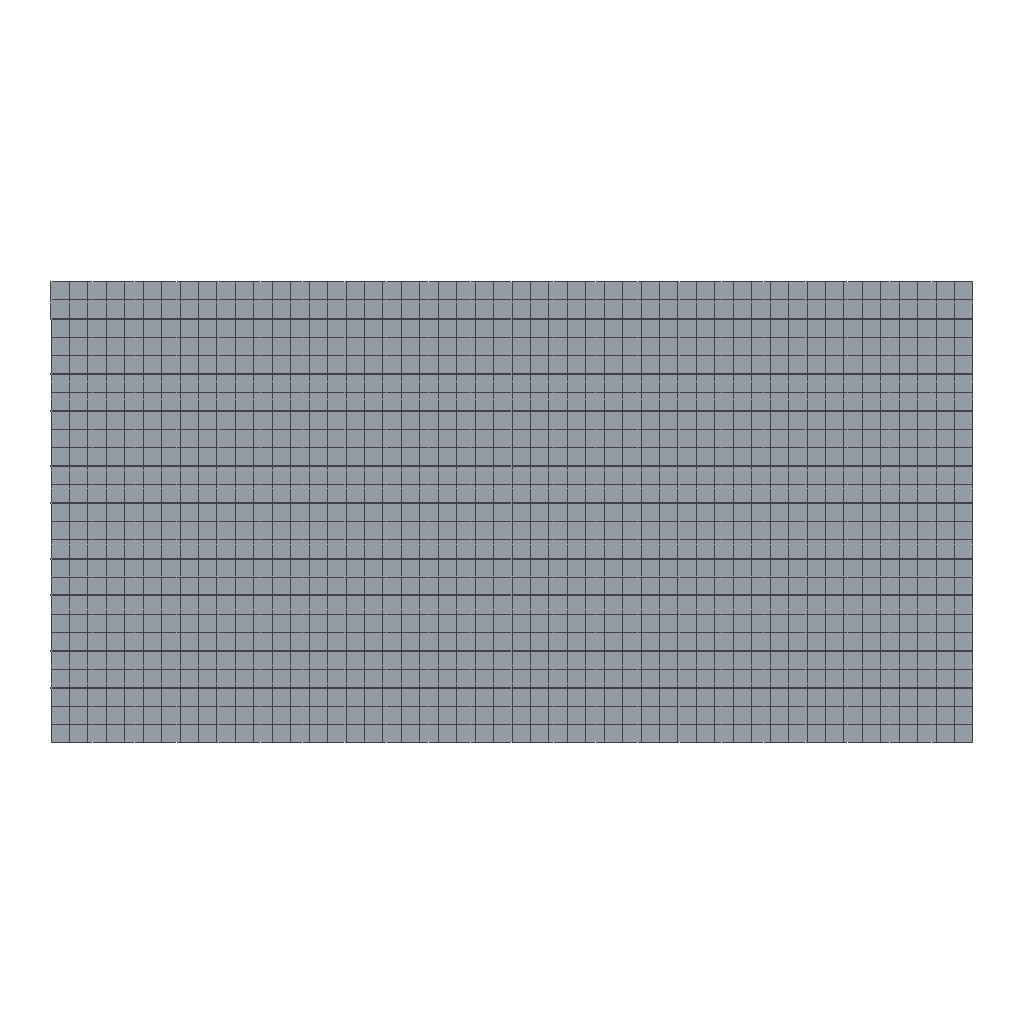Simulation study | abaqus
Set-up summary:
category,name,step,type,value,unit,region
solver,abaqus
solver,version,,,Abaqus/Explicit 2020
units,not stated in the deck,,not stated
analysis,deck,,transient,transient
load_step,Step-1,Step-1,transient
load_step,requested,,,1
mesh,nodes,,,2353
mesh,elements,,,1610
element_type,CPS4R,,plane,1250
element_type,COH2D4,,cohesive,360
load,load commands in deck,,count,1
bc,support commands in deck,,count,4
material,MATERIAL-3,,in results
material,SIC,,in results
material,T300,,in results
check,setup vs results,,match,"per instance, exact: element labels, types and connectivity; labels of the nodes the elements use; coordinates of those nodes at DOUBLE_PRECISION in 1 of 4 instance(s)"
Abaqus input file, long lists of numbers shortened:
*Heading
** Job name: Job-3 Model name: Model-1-Copy
** Generated by: Abaqus/CAE 2020
*Preprint, echo=NO, model=NO, history=NO, contact=NO
**
** PARTS
**
*Part, name=coh
*Node
      1, -0.1, -0.038
      2, -0.1, -0.0382
** (565 more lines like these left out)
*Element, type=COH2D4
 1,   1,  37, 397,  76
 2,  37,   2,  38, 397
** (358 more lines like these left out)
*Nset, nset=Set-1, generate
   1,  567,    1
*Elset, elset=Set-1, generate
   1,  360,    1
** Section: coh
*Cohesive Section, elset=Set-1, controls=EC-1, material=Material-3, response=TRACTION SEPARATION
,
*End Part
**
*Part, name=lay-1
*Node
      1, -0.1, 0.05
      2, -0.1, 0.046
** (151 more lines like these left out)
*Element, type=CPS4R
  1,   1,   2,   5,   4
  2,   2,   3,   6,   5
** (98 more lines like these left out)
*Nset, nset=Set-3, generate
   1,  153,    1
*Elset, elset=Set-3, generate
   1,  100,    1
*Orientation, name=Ori-1
1., 0., 0., 0., 1., 0.
3, 0.
** Section: t300
*Solid Section, elset=Set-3, orientation=Ori-1, material=t300
,
*End Part
**
*Part, name=rigid
*End Part
**
*Part, name=work
*Node
      1,  0.2, -0.0882
      2,           0., -0.0882
** (1630 more lines like these left out)
*Element, type=CPS4R
  1,    1,   37,  947,  138
  2,   37,   38,  948,  947
** (1148 more lines like these left out)
*Nset, nset=Set-2
   29,   30,   31,   32,  743,  744,  745,  746,  747,  748,  749,  750,  751,  752,  753,  754
  755,  756,  757,  758,  759,  760,  761,  762,  763,  764,  765,  766,  767,  768,  769,  770
** (11 more lines like these left out)
*Elset, elset=Set-2, generate
  851,  1000,     1
*Nset, nset=Set-3
   21,   22,   23,   24,  543,  544,  545,  546,  547,  548,  549,  550,  551,  552,  553,  554
  555,  556,  557,  558,  559,  560,  561,  562,  563,  564,  565,  566,  567,  568,  569,  570
** (8 more lines like these left out)
*Elset, elset=Set-3, generate
 651,  750,    1
*Nset, nset=Set-4
   13,   14,   15,   16,  341,  342,  343,  344,  345,  346,  347,  348,  349,  350,  351,  352
  353,  354,  355,  356,  357,  358,  359,  360,  361,  362,  363,  364,  365,  366,  367,  368
** (11 more lines like these left out)
*Elset, elset=Set-4, generate
 401,  550,    1
*Nset, nset=Set-6
    5,    6,    7,    8,  139,  140,  141,  142,  143,  144,  145,  146,  147,  148,  149,  150
  151,  152,  153,  154,  155,  156,  157,  158,  159,  160,  161,  162,  163,  164,  165,  166
** (8 more lines like these left out)
*Elset, elset=Set-6, generate
 151,  250,    1
*Nset, nset=Set-7
    1,    2,    3,    4,    9,   10,   11,   12,   17,   18,   19,   20,   25,   26,   27,   28
   33,   34,   35,   36,   37,   38,   39,   40,   41,   42,   43,   44,   45,   46,   47,   48
** (56 more lines like these left out)
*Elset, elset=Set-7
    1,    2,    3,    4,    5,    6,    7,    8,    9,   10,   11,   12,   13,   14,   15,   16
   17,   18,   19,   20,   21,   22,   23,   24,   25,   26,   27,   28,   29,   30,   31,   32
** (39 more lines like these left out)
*Nset, nset=Set-18
    5,    6,    7,    8,   17,   18,   19,   20,   21,   22,   23,   24,   25,   26,   27,   28
  139,  140,  141,  142,  143,  144,  145,  146,  147,  148,  149,  150,  151,  152,  153,  154
** (37 more lines like these left out)
*Elset, elset=Set-18
 151, 152, 153, 154, 155, 156, 157, 158, 159, 160, 161, 162, 163, 164, 165, 166
 167, 168, 169, 170, 171, 172, 173, 174, 175, 176, 177, 178, 179, 180, 181, 182
** (23 more lines like these left out)
*Nset, nset=Set-19
    1,    2,    3,    4,    9,   10,   11,   12,   13,   14,   15,   16,   29,   30,   31,   32
   33,   34,   35,   36,   37,   38,   39,   40,   41,   42,   43,   44,   45,   46,   47,   48
** (62 more lines like these left out)
*Elset, elset=Set-19
    1,    2,    3,    4,    5,    6,    7,    8,    9,   10,   11,   12,   13,   14,   15,   16
   17,   18,   19,   20,   21,   22,   23,   24,   25,   26,   27,   28,   29,   30,   31,   32
** (45 more lines like these left out)
** Section: sic
*Solid Section, elset=Set-19, material=sic
,
*Orientation, name=Ori-2
1., 0., 0., 0., 1., 0.
3, 0.
** Section: t300
*Solid Section, elset=Set-18, orientation=Ori-2, material=t300
,
*End Part
**
**
** ASSEMBLY
**
*Assembly, name=Assembly
**
*Instance, name=rigid-1, part=rigid
    0.2142,     0.001757,           0.
*Node
      1, 0.005757, -0.01114,           0.
*Nset, nset=rigid-1-RefPt_, internal
1,
*Surface, type=SEGMENTS, name=m_Surf-1
START, 0.01, -0.01
 CIRCL, 0.001515, -0.01, 0.005757, -0.002652
 LINE, -0.04179,        0.015
 LINE, 0.0533,        0.015
 LINE, 0.01, -0.01
*Rigid Body, ref node=rigid-1-RefPt_, analytical surface=m_Surf-1
*End Instance
**
*Instance, name=work-1, part=work
*End Instance
**
*Instance, name=coh-1, part=coh
         0.1,        -0.05,           0.
*End Instance
**
*Instance, name=lay-1-1, part=lay-1
         0.1,        -0.05,           0.
*End Instance
**
*Nset, nset=Set-2, instance=work-1
   3,   4,  88,  89,  90,  91,  92,  93,  94,  95,  96,  97,  98,  99, 100, 101
 102, 103, 104, 105, 106, 107, 108, 109, 110, 111, 112, 113, 114, 115, 116, 117
** (2 more lines like these left out)
*Elset, elset=Set-2, instance=work-1, generate
 101,  150,    1
*Nset, nset=Set-3, instance=work-1
   1,   3,   4,  14,  15,  21,  24,  88,  89,  90,  91,  92,  93,  94,  95,  96
  97,  98,  99, 100, 101, 102, 103, 104, 105, 106, 107, 108, 109, 110, 111, 112
** (2 more lines like these left out)
*Elset, elset=Set-3, instance=work-1
   1,  51, 101, 102, 103, 104, 105, 106, 107, 108, 109, 110, 111, 112, 113, 114
 115, 116, 117, 118, 119, 120, 121, 122, 123, 124, 125, 126, 127, 128, 129, 130
** (2 more lines like these left out)
*Nset, nset=Set-4, instance=rigid-1
 1,
*Nset, nset=Set-5, instance=rigid-1
 1,
*Nset, nset=Set-6, instance=work-1
   1,   2,   3,   4,   5,   6,   7,   8,   9,  10,  11,  12,  13,  14,  15,  16
  17,  18,  19,  20,  21,  22,  23,  24,  25,  26,  27,  28,  33,  34,  35,  36
** (5 more lines like these left out)
*Nset, nset=Set-6, instance=coh-1
   1,   2,   3,   4,   5,   6,   7,   8,   9,  10,  11,  12,  13,  14,  15,  16
  21,  22,  23,  24,  25,  26,  27,  28,  29,  30,  31,  32,  37,  57,  77,  97
** (1 more lines like these left out)
*Elset, elset=Set-6, instance=work-1
    1,   50,   51,  100,  101,  102,  103,  104,  105,  106,  107,  108,  109,  110,  111,  112
  113,  114,  115,  116,  117,  118,  119,  120,  121,  122,  123,  124,  125,  126,  127,  128
** (4 more lines like these left out)
*Elset, elset=Set-6, instance=coh-1
   1,   2,  39,  40,  41,  42,  79,  80,  81,  82, 119, 120, 121, 122, 159, 160
 201, 202, 239, 240, 241, 242, 279, 280, 281, 282, 319, 320
*Nset, nset=s_Set-1, instance=work-1
   29,   30,   31,   32,  743,  744,  745,  746,  747,  748,  749,  750,  751,  752,  753,  754
  755,  756,  757,  758,  759,  760,  761,  762,  763,  764,  765,  766,  767,  768,  769,  770
** (11 more lines like these left out)
*Elset, elset=s_Set-1, instance=work-1, generate
  851,  1000,     1
*Nset, nset=s_Set-7, instance=work-1
   29,   30,   31,   32,  743,  744,  745,  746,  747,  748,  749,  750,  751,  752,  753,  754
  755,  756,  757,  758,  759,  760,  761,  762,  763,  764,  765,  766,  767,  768,  769,  770
** (11 more lines like these left out)
*Nset, nset=s_Set-7, instance=coh-1
  17,  18,  19,  20, 197, 198, 199, 200, 201, 202, 203, 204, 205, 206, 207, 208
 209, 210, 211, 212, 213, 214, 215, 216, 217, 218, 219, 220, 221, 222, 223, 224
** (2 more lines like these left out)
*Elset, elset=s_Set-7, instance=work-1, generate
  851,  1000,     1
*Elset, elset=s_Set-7, instance=coh-1, generate
 161,  200,    1
*Nset, nset=s_Set-8, instance=work-1
   29,   30,   31,   32,  743,  744,  745,  746,  747,  748,  749,  750,  751,  752,  753,  754
  755,  756,  757,  758,  759,  760,  761,  762,  763,  764,  765,  766,  767,  768,  769,  770
** (11 more lines like these left out)
*Nset, nset=s_Set-8, instance=coh-1
  17,  18,  19,  20, 197, 198, 199, 200, 201, 202, 203, 204, 205, 206, 207, 208
 209, 210, 211, 212, 213, 214, 215, 216, 217, 218, 219, 220, 221, 222, 223, 224
** (2 more lines like these left out)
*Nset, nset=s_Set-8, instance=lay-1-1, generate
   1,  153,    1
*Elset, elset=s_Set-8, instance=work-1, generate
  851,  1000,     1
*Elset, elset=s_Set-8, instance=coh-1, generate
 161,  200,    1
*Elset, elset=s_Set-8, instance=lay-1-1, generate
   1,  100,    1
*Nset, nset=s_Set-9, instance=lay-1-1, generate
   1,  153,    1
*Elset, elset=s_Set-9, instance=lay-1-1, generate
   1,  100,    1
*Nset, nset=s_Set-10, instance=work-1
   29,   30,   31,   32,  743,  744,  745,  746,  747,  748,  749,  750,  751,  752,  753,  754
  755,  756,  757,  758,  759,  760,  761,  762,  763,  764,  765,  766,  767,  768,  769,  770
** (11 more lines like these left out)
*Elset, elset=s_Set-10, instance=work-1, generate
  851,  1000,     1
*Elset, elset=_m_Surf-2_S1, internal, instance=coh-1
   1,   2,  41,  42,  81,  82, 121, 122, 161, 162, 201, 202, 241, 242, 281, 282
 321, 322
*Elset, elset=_m_Surf-2_S2, internal, instance=coh-1, generate
   2,  360,    2
*Elset, elset=_m_Surf-2_S3, internal, instance=coh-1
  39,  40,  79,  80, 119, 120, 159, 160, 199, 200, 239, 240, 279, 280, 319, 320
 359, 360
*Elset, elset=_m_Surf-2_S4, internal, instance=coh-1, generate
   1,  359,    2
*Surface, type=ELEMENT, name=m_Surf-2
_m_Surf-2_S1, S1
_m_Surf-2_S2, S2
_m_Surf-2_S4, S4
_m_Surf-2_S3, S3
*Elset, elset=_m_Surf-6_S4, internal, instance=coh-1, generate
 161,  199,    2
*Surface, type=ELEMENT, name=m_Surf-6
_m_Surf-6_S4, S4
*Elset, elset=_m_Surf-8_S2, internal, instance=coh-1, generate
 162,  200,    2
*Surface, type=ELEMENT, name=m_Surf-8
_m_Surf-8_S2, S2
*Elset, elset=_m_Surf-10_S4, internal, instance=coh-1, generate
 321,  359,    2
*Surface, type=ELEMENT, name=m_Surf-10
_m_Surf-10_S4, S4
*Elset, elset=_m_Surf-12_S2, internal, instance=coh-1, generate
 322,  360,    2
*Surface, type=ELEMENT, name=m_Surf-12
_m_Surf-12_S2, S2
*Elset, elset=_m_Surf-14_S4, internal, instance=coh-1, generate
 121,  159,    2
*Surface, type=ELEMENT, name=m_Surf-14
_m_Surf-14_S4, S4
*Elset, elset=_m_Surf-16_S2, internal, instance=coh-1, generate
 122,  160,    2
*Surface, type=ELEMENT, name=m_Surf-16
_m_Surf-16_S2, S2
*Elset, elset=_m_Surf-18_S4, internal, instance=coh-1, generate
 281,  319,    2
*Surface, type=ELEMENT, name=m_Surf-18
_m_Surf-18_S4, S4
*Elset, elset=_m_Surf-20_S2, internal, instance=coh-1, generate
 282,  320,    2
*Surface, type=ELEMENT, name=m_Surf-20
_m_Surf-20_S2, S2
*Elset, elset=_m_Surf-22_S4, internal, instance=coh-1, generate
  81,  119,    2
*Surface, type=ELEMENT, name=m_Surf-22
_m_Surf-22_S4, S4
*Elset, elset=_m_Surf-24_S2, internal, instance=coh-1, generate
  82,  120,    2
*Surface, type=ELEMENT, name=m_Surf-24
_m_Surf-24_S2, S2
*Elset, elset=_m_Surf-26_S4, internal, instance=coh-1, generate
 241,  279,    2
*Surface, type=ELEMENT, name=m_Surf-26
_m_Surf-26_S4, S4
*Elset, elset=_m_Surf-28_S2, internal, instance=coh-1, generate
 242,  280,    2
*Surface, type=ELEMENT, name=m_Surf-28
_m_Surf-28_S2, S2
*Elset, elset=_m_Surf-30_S4, internal, instance=coh-1, generate
 41,  79,   2
*Surface, type=ELEMENT, name=m_Surf-30
_m_Surf-30_S4, S4
*Elset, elset=_m_Surf-32_S2, internal, instance=coh-1, generate
 42,  80,   2
*Surface, type=ELEMENT, name=m_Surf-32
_m_Surf-32_S2, S2
*Elset, elset=_m_Surf-34_S4, internal, instance=coh-1, generate
 201,  239,    2
*Surface, type=ELEMENT, name=m_Surf-34
_m_Surf-34_S4, S4
*Elset, elset=_m_Surf-36_S2, internal, instance=coh-1, generate
 202,  240,    2
*Surface, type=ELEMENT, name=m_Surf-36
_m_Surf-36_S2, S2
*Elset, elset=_m_Surf-38_S4, internal, instance=coh-1, generate
  1,  39,   2
*Surface, type=ELEMENT, name=m_Surf-38
_m_Surf-38_S4, S4
*Elset, elset=_m_Surf-40_S2, internal, instance=coh-1, generate
  2,  40,   2
*Surface, type=ELEMENT, name=m_Surf-40
_m_Surf-40_S2, S2
*Elset, elset=_m_Surf-42_S2, internal, instance=lay-1-1, generate
   2,  100,    2
*Surface, type=ELEMENT, name=m_Surf-42
_m_Surf-42_S2, S2
*Elset, elset=_s_Surf-2_S1, internal, instance=work-1
    1,    2,    3,    4,    5,    6,    7,    8,    9,   10,   11,   12,   13,   14,   15,   16
   17,   18,   19,   20,   21,   22,   23,   24,   25,   26,   27,   28,   29,   30,   31,   32
** (27 more lines like these left out)
*Elset, elset=_s_Surf-2_S3, internal, instance=work-1
  201,  202,  203,  204,  205,  206,  207,  208,  209,  210,  211,  212,  213,  214,  215,  216
  217,  218,  219,  220,  221,  222,  223,  224,  225,  226,  227,  228,  229,  230,  231,  232
** (23 more lines like these left out)
*Surface, type=ELEMENT, name=s_Surf-2
_s_Surf-2_S1, S1
_s_Surf-2_S3, S3
*Elset, elset=_s_Surf-4_S3, internal, instance=work-1
  701,  702,  703,  704,  705,  706,  707,  708,  709,  710,  711,  712,  713,  714,  715,  716
  717,  718,  719,  720,  721,  722,  723,  724,  725,  726,  727,  728,  729,  730,  731,  732
** (5 more lines like these left out)
*Elset, elset=_s_Surf-4_S3, internal, instance=coh-1
 199, 200, 359, 360
*Elset, elset=_s_Surf-4_S1, internal, instance=work-1, generate
 851,  900,    1
*Elset, elset=_s_Surf-4_S1, internal, instance=coh-1
 161, 162
*Elset, elset=_s_Surf-4_S2, internal, instance=work-1, generate
  900,  1000,    50
*Elset, elset=_s_Surf-4_S2, internal, instance=coh-1
 162, 164, 166, 168, 170, 172, 174, 176, 178, 180, 182, 184, 186, 188, 190, 192
 194, 196, 198, 200, 322, 324, 326, 328, 330, 332, 334, 336, 338, 340, 342, 344
** (1 more lines like these left out)
*Elset, elset=_s_Surf-4_S4, internal, instance=work-1, generate
 851,  951,   50
*Elset, elset=_s_Surf-4_S4, internal, instance=coh-1
 161, 163, 165, 167, 169, 171, 173, 175, 177, 179, 181, 183, 185, 187, 189, 191
 193, 195, 197, 199, 321, 323, 325, 327, 329, 331, 333, 335, 337, 339, 341, 343
** (1 more lines like these left out)
*Surface, type=ELEMENT, name=s_Surf-4
_s_Surf-4_S3, S3
_s_Surf-4_S1, S1
_s_Surf-4_S2, S2
_s_Surf-4_S4, S4
*Elset, elset=_s_Surf-8_S3, internal, instance=work-1, generate
  951,  1000,     1
*Surface, type=ELEMENT, name=s_Surf-8
_s_Surf-8_S3, S3
*Elset, elset=_s_Surf-10_S1, internal, instance=work-1, generate
 851,  900,    1
*Surface, type=ELEMENT, name=s_Surf-10
_s_Surf-10_S1, S1
*Elset, elset=_s_Surf-12_S3, internal, instance=work-1, generate
 701,  750,    1
*Surface, type=ELEMENT, name=s_Surf-12
_s_Surf-12_S3, S3
*Elset, elset=_s_Surf-14_S1, internal, instance=work-1, generate
 651,  700,    1
*Surface, type=ELEMENT, name=s_Surf-14
_s_Surf-14_S1, S1
*Elset, elset=_s_Surf-16_S1, internal, instance=work-1, generate
 401,  450,    1
*Surface, type=ELEMENT, name=s_Surf-16
_s_Surf-16_S1, S1
*Elset, elset=_s_Surf-18_S3, internal, instance=work-1, generate
 501,  550,    1
*Surface, type=ELEMENT, name=s_Surf-18
_s_Surf-18_S3, S3
*Elset, elset=_s_Surf-20_S1, internal, instance=work-1, generate
 151,  200,    1
*Surface, type=ELEMENT, name=s_Surf-20
_s_Surf-20_S1, S1
*Elset, elset=_s_Surf-22_S3, internal, instance=work-1, generate
 201,  250,    1
*Surface, type=ELEMENT, name=s_Surf-22
_s_Surf-22_S3, S3
*Elset, elset=_s_Surf-24_S3, internal, instance=work-1, generate
 351,  400,    1
*Surface, type=ELEMENT, name=s_Surf-24
_s_Surf-24_S3, S3
*Elset, elset=_s_Surf-26_S1, internal, instance=work-1, generate
 251,  300,    1
*Surface, type=ELEMENT, name=s_Surf-26
_s_Surf-26_S1, S1
*Elset, elset=_s_Surf-28_S3, internal, instance=work-1, generate
 801,  850,    1
*Surface, type=ELEMENT, name=s_Surf-28
_s_Surf-28_S3, S3
*Elset, elset=_s_Surf-30_S1, internal, instance=work-1, generate
 751,  800,    1
*Surface, type=ELEMENT, name=s_Surf-30
_s_Surf-30_S1, S1
*Elset, elset=_s_Surf-32_S1, internal, instance=work-1, generate
 1001,  1050,     1
*Surface, type=ELEMENT, name=s_Surf-32
_s_Surf-32_S1, S1
*Elset, elset=_s_Surf-34_S3, internal, instance=work-1, generate
 1101,  1150,     1
*Surface, type=ELEMENT, name=s_Surf-34
_s_Surf-34_S3, S3
*Elset, elset=_s_Surf-36_S1, internal, instance=work-1, generate
 551,  600,    1
*Surface, type=ELEMENT, name=s_Surf-36
_s_Surf-36_S1, S1
*Elset, elset=_s_Surf-38_S3, internal, instance=work-1, generate
 601,  650,    1
*Surface, type=ELEMENT, name=s_Surf-38
_s_Surf-38_S3, S3
*Elset, elset=_s_Surf-40_S1, internal, instance=work-1, generate
  1,  50,   1
*Surface, type=ELEMENT, name=s_Surf-40
_s_Surf-40_S1, S1
*Elset, elset=_s_Surf-42_S4, internal, instance=coh-1, generate
 161,  199,    2
*Surface, type=ELEMENT, name=s_Surf-42
_s_Surf-42_S4, S4
*Elset, elset=_s_Surf-44_S2, internal, instance=coh-1, generate
 162,  200,    2
*Surface, type=ELEMENT, name=s_Surf-44
_s_Surf-44_S2, S2
*Elset, elset=_s_Surf-46_S2, internal, instance=work-1, generate
  900,  1000,    50
*Surface, type=ELEMENT, name=s_Surf-46
_s_Surf-46_S2, S2
*Surface, type=NODE, name=s_Set-9_CNS_, internal
s_Set-9, 1.
*Surface, type=NODE, name=s_Set-10_CNS_, internal
s_Set-10, 1.
** Constraint: Constraint-2
*Tie, name=Constraint-2, adjust=yes
s_Surf-42, m_Surf-42
** Constraint: Constraint-3
*Tie, name=Constraint-3, adjust=yes
s_Surf-8, m_Surf-8
** Constraint: Constraint-4
*Tie, name=Constraint-4, adjust=yes
s_Surf-10, m_Surf-10
** Constraint: Constraint-5
*Tie, name=Constraint-5, adjust=yes
s_Surf-12, m_Surf-12
** Constraint: Constraint-6
*Tie, name=Constraint-6, adjust=yes
s_Surf-14, m_Surf-14
** Constraint: Constraint-7
*Tie, name=Constraint-7, adjust=yes
s_Surf-16, m_Surf-16
** Constraint: Constraint-8
*Tie, name=Constraint-8, adjust=yes
s_Surf-18, m_Surf-18
** Constraint: Constraint-9
*Tie, name=Constraint-9, adjust=yes
s_Surf-20, m_Surf-20
** Constraint: Constraint-10
*Tie, name=Constraint-10, adjust=yes
s_Surf-22, m_Surf-22
** Constraint: Constraint-11
*Tie, name=Constraint-11, adjust=yes
s_Surf-24, m_Surf-24
** Constraint: Constraint-12
*Tie, name=Constraint-12, adjust=yes
s_Surf-26, m_Surf-26
** Constraint: Constraint-13
*Tie, name=Constraint-13, adjust=yes
s_Surf-28, m_Surf-28
** Constraint: Constraint-14
*Tie, name=Constraint-14, adjust=yes
s_Surf-30, m_Surf-30
** Constraint: Constraint-15
*Tie, name=Constraint-15, adjust=yes
s_Surf-32, m_Surf-32
** Constraint: Constraint-16
*Tie, name=Constraint-16, adjust=yes
s_Surf-34, m_Surf-34
** Constraint: Constraint-17
*Tie, name=Constraint-17, adjust=yes
s_Surf-36, m_Surf-36
** Constraint: Constraint-18
*Tie, name=Constraint-18, adjust=yes
s_Surf-38, m_Surf-38
** Constraint: Constraint-19
*Tie, name=Constraint-19, adjust=yes
s_Surf-40, m_Surf-40
*End Assembly
**
** ELEMENT CONTROLS
**
*Section Controls, name=EC-1, ELEMENT DELETION=YES
1., 1., 1.
*Amplitude, name=Amp-1
             0.,              0.,          0.0026,              1.
**
** MATERIALS
**
*Material, name=Material-3
*Damage Initiation, criterion=QUADE
 1e-05, 1e-05, 1e-05
*Damage Evolution, type=DISPLACEMENT
 1e-09,
*Density
 2e-09,
*Elastic, type=TRACTION
70000.,20000.,20000.
*Material, name=sic
*Density
 3.22e-09,
*Elastic
36600., 0.15
*Plastic
355.,0.
*Material, name=t300
*Density
 1.76e-09,
*Elastic, type=LAMINA
15000.,250000.,    0.2, 15000., 15000.,  7000.
**
** INTERACTION PROPERTIES
**
*Surface Interaction, name=IntProp-1
*Friction
 0.2,
*Surface Behavior, pressure-overclosure=HARD
**
** INTERACTIONS
**
** Interaction: Int-2
*Contact, op=NEW
*Contact Inclusions, ALL EXTERIOR
*Contact Property Assignment
 ,  , IntProp-1
** ----------------------------------------------------------------
**
** STEP: Step-1
**
*Step, name=Step-1, nlgeom=YES
*Dynamic, Explicit
, 0.0026
*Bulk Viscosity
0.06, 1.2
** Mass Scaling: Semi-Automatic
**               Whole Model
*Fixed Mass Scaling, factor=500.
**
** BOUNDARY CONDITIONS
**
** Name: BC-1 Type: 对称/反对称/完全固定
*Boundary
Set-6, ENCASTRE
** Name: BC-2 Type: 速度/角速度
*Boundary, type=VELOCITY
Set-4, 1, 1, -83.
Set-4, 2, 2
Set-4, 6, 6
**
** INTERACTIONS
**
** Interaction: Int-6
*Contact Pair, interaction=IntProp-1, mechanical constraint=KINEMATIC, cpset=Int-6
rigid-1.m_Surf-1, s_Set-9_CNS_
** Interaction: Int-7
*Contact Pair, interaction=IntProp-1, mechanical constraint=KINEMATIC, cpset=Int-7
rigid-1.m_Surf-1, s_Set-10_CNS_
**
** OUTPUT REQUESTS
**
*Restart, write, number interval=1, time marks=NO
**
** FIELD OUTPUT: F-Output-1
**
*Output, field, number interval=50
*Node Output
CF, RF, U, V
*Element Output, directions=YES
E, LE, MISES, MISESMAX, PE, PEEQ, PEMAG, S, SDEG, STATUS, TSHR
*Contact Output
CDISP, CSDMG, CSTRESS
**
** HISTORY OUTPUT: H-Output-1
**
*Output, history, variable=PRESELECT, frequency=10
*End Step
Results summary:
result,step,Step-1,completed,increments=713552 time=0.0026/0.0026
result,analysis,,,transient
result,last_loadstep,,,1
result,primary field,,,U
result,reaction total,,FX,-29.816,model units
result,reaction total,,FY,-37.15,model units
result,reaction total,,FZ,0.0,model units